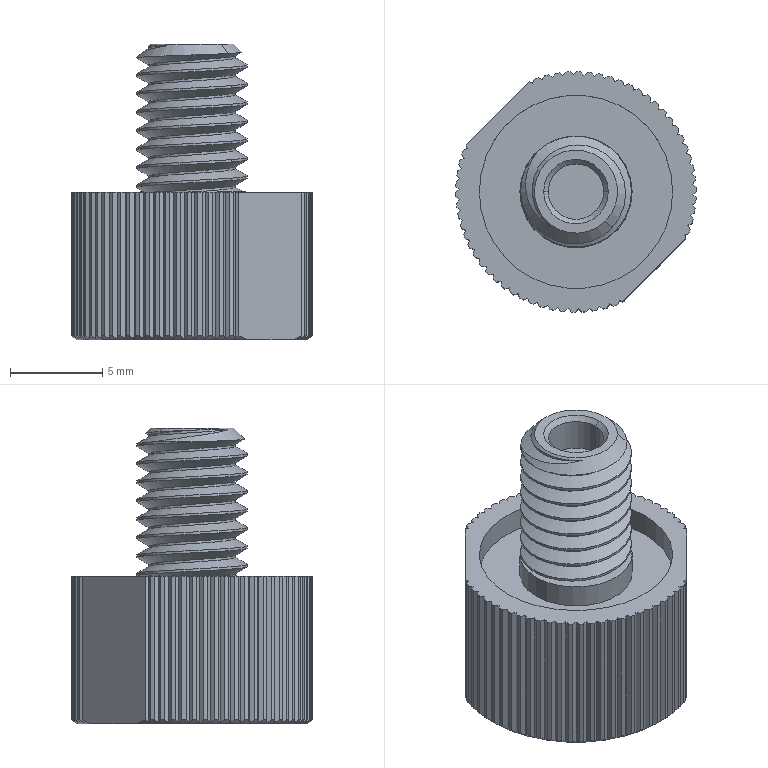Part | SolidWorks | features ICE 51, HoleWzd 2, BaseBody 1, Chamfer 1 | 1 solid | 204 faces | box 13 x 13 x 16 mm | volume 1107 mm3 | plane 117 | cylinder 76 | cone 8 | spline 3 | commonest cylinder face diameters 13 x52 6 x16 3 x4 6.07 x2 10.45 x2